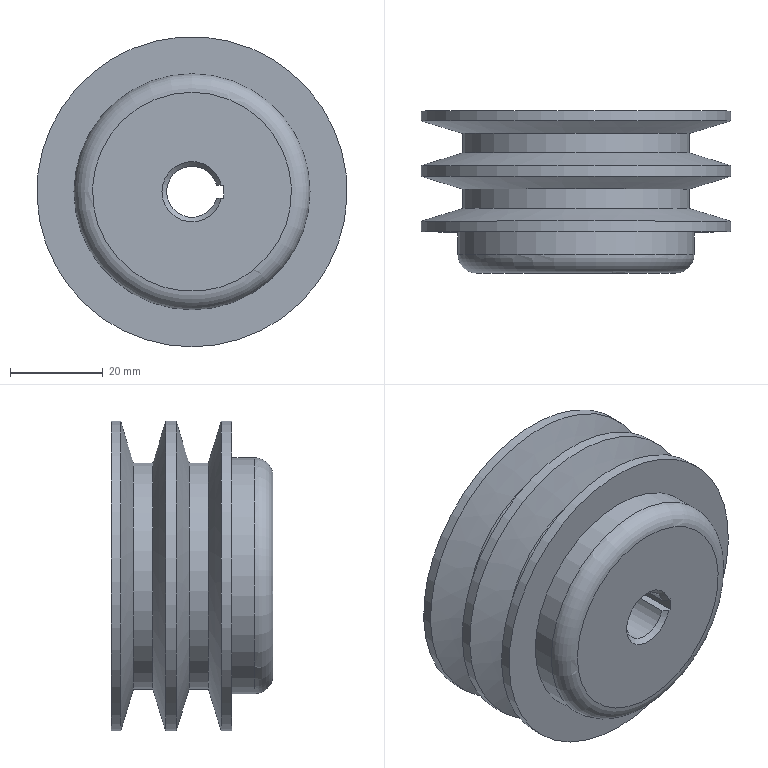Part | NX | features DATUM_CSYS 3, SKETCH 2, BLEND 1, CHAMFER 1, EXTRUDE 1, SWP104 1 | 1 solid | 20 faces | box 67 x 35 x 67 mm | volume 82909 mm3 | cylinder 7 | plane 6 | cone 6 | torus 1 | commonest cylinder face diameters 67 x3 49 x2 11 x1 51 x1
STEP:
#1=CARTESIAN_POINT('',(0.,0.,21.5));
#2=VERTEX_POINT('',#1);
#3=CARTESIAN_POINT('',(0.,0.,0.));
#4=DIRECTION('',(0.,1.,0.));
#5=DIRECTION('',(0.,0.,1.));
#6=AXIS2_PLACEMENT_3D('',#3,#4,#5);
#7=CIRCLE('',#6,21.5);
#8=EDGE_CURVE('',#2,#2,#7,.F.);
#9=ORIENTED_EDGE('',*,*,#8,.T.);
#10=EDGE_LOOP('',(#9));
#11=FACE_BOUND('',#10,.T.);
#12=CARTESIAN_POINT('',(6.347,0.,-1.4));
#13=VERTEX_POINT('',#12);
#14=CARTESIAN_POINT('',(6.9,0.,-1.4));
#15=VERTEX_POINT('',#14);
#16=CARTESIAN_POINT('',(0.,0.,-1.4));
#17=DIRECTION('',(1.,0.,0.));
#18=VECTOR('',#17,1000.);
#19=LINE('',#16,#18);
#20=EDGE_CURVE('',#13,#15,#19,.T.);
#21=ORIENTED_EDGE('',*,*,#20,.F.);
#22=CARTESIAN_POINT('',(6.347,0.,1.4));
#23=VERTEX_POINT('',#22);
#24=CARTESIAN_POINT('',(0.,0.,0.));
#25=DIRECTION('',(0.,1.,0.));
#26=DIRECTION('',(0.,0.,1.));
#27=AXIS2_PLACEMENT_3D('',#24,#25,#26);
#28=CIRCLE('',#27,6.5);
#29=EDGE_CURVE('',#13,#23,#28,.T.);
#30=ORIENTED_EDGE('',*,*,#29,.T.);
#31=CARTESIAN_POINT('',(6.9,0.,1.4));
#32=VERTEX_POINT('',#31);
#33=CARTESIAN_POINT('',(0.,0.,1.4));
#34=DIRECTION('',(-1.,0.,0.));
#35=VECTOR('',#34,1000.);
#36=LINE('',#33,#35);
#37=EDGE_CURVE('',#32,#23,#36,.T.);
#38=ORIENTED_EDGE('',*,*,#37,.F.);
#39=CARTESIAN_POINT('',(6.9,0.,25.5));
#40=DIRECTION('',(0.,0.,1.));
#41=VECTOR('',#40,1000.);
#42=LINE('',#39,#41);
#43=EDGE_CURVE('',#15,#32,#42,.T.);
#44=ORIENTED_EDGE('',*,*,#43,.F.);
#45=EDGE_LOOP('',(#21,#30,#38,#44));
#46=FACE_BOUND('',#45,.T.);
#47=CARTESIAN_POINT('',(0.,0.,25.5));
#48=DIRECTION('',(0.,1.,0.));
#49=DIRECTION('',(0.,0.,1.));
#50=AXIS2_PLACEMENT_3D('',#47,#48,#49);
#51=PLANE('',#50);
#52=ADVANCED_FACE('',(#11,#46),#51,.F.);
#53=CARTESIAN_POINT('',(5.319,34.,-1.4));
#54=VERTEX_POINT('',#53);
#55=CARTESIAN_POINT('',(5.319,1.,-1.4));
#56=VERTEX_POINT('',#55);
#57=CARTESIAN_POINT('',(5.319,0.,-1.4));
#58=DIRECTION('',(0.,-1.,0.));
#59=VECTOR('',#58,1000.);
#60=LINE('',#57,#59);
#61=EDGE_CURVE('',#54,#56,#60,.T.);
#62=ORIENTED_EDGE('',*,*,#61,.F.);
#63=CARTESIAN_POINT('',(5.319,34.,1.4));
#64=VERTEX_POINT('',#63);
#65=CARTESIAN_POINT('',(0.,34.,0.));
#66=DIRECTION('',(0.,-1.,0.));
#67=DIRECTION('',(0.,0.,-1.));
#68=AXIS2_PLACEMENT_3D('',#65,#66,#67);
#69=CIRCLE('',#68,5.5);
#70=EDGE_CURVE('',#54,#64,#69,.F.);
#71=ORIENTED_EDGE('',*,*,#70,.T.);
#72=CARTESIAN_POINT('',(5.319,1.,1.4));
#73=VERTEX_POINT('',#72);
#74=CARTESIAN_POINT('',(5.319,0.,1.4));
#75=DIRECTION('',(0.,-1.,0.));
#76=VECTOR('',#75,1000.);
#77=LINE('',#74,#76);
#78=EDGE_CURVE('',#73,#64,#77,.F.);
#79=ORIENTED_EDGE('',*,*,#78,.F.);
#80=CARTESIAN_POINT('',(0.,1.,0.));
#81=DIRECTION('',(0.,1.,0.));
#82=DIRECTION('',(0.,0.,1.));
#83=AXIS2_PLACEMENT_3D('',#80,#81,#82);
#84=CIRCLE('',#83,5.5);
#85=EDGE_CURVE('',#73,#56,#84,.F.);
#86=ORIENTED_EDGE('',*,*,#85,.T.);
#87=EDGE_LOOP('',(#62,#71,#79,#86));
#88=FACE_BOUND('',#87,.T.);
#89=CARTESIAN_POINT('',(0.,0.,0.));
#90=DIRECTION('',(0.,-1.,0.));
#91=DIRECTION('',(0.,0.,-1.));
#92=AXIS2_PLACEMENT_3D('',#89,#90,#91);
#93=CYLINDRICAL_SURFACE('',#92,5.5);
#94=ADVANCED_FACE('',(#88),#93,.F.);
#95=CARTESIAN_POINT('',(0.,35.,-33.5));
#96=VERTEX_POINT('',#95);
#97=CARTESIAN_POINT('',(0.,35.,0.));
#98=DIRECTION('',(0.,-1.,0.));
#99=DIRECTION('',(0.,0.,-1.));
#100=AXIS2_PLACEMENT_3D('',#97,#98,#99);
#101=CIRCLE('',#100,33.5);
#102=EDGE_CURVE('',#96,#96,#101,.T.);
#103=ORIENTED_EDGE('',*,*,#102,.F.);
#104=EDGE_LOOP('',(#103));
#105=FACE_BOUND('',#104,.T.);
#106=CARTESIAN_POINT('',(6.347,35.,1.4));
#107=VERTEX_POINT('',#106);
#108=CARTESIAN_POINT('',(6.9,35.,1.4));
#109=VERTEX_POINT('',#108);
#110=CARTESIAN_POINT('',(0.,35.,1.4));
#111=DIRECTION('',(1.,0.,0.));
#112=VECTOR('',#111,1000.);
#113=LINE('',#110,#112);
#114=EDGE_CURVE('',#107,#109,#113,.T.);
#115=ORIENTED_EDGE('',*,*,#114,.F.);
#116=CARTESIAN_POINT('',(6.347,35.,-1.4));
#117=VERTEX_POINT('',#116);
#118=CARTESIAN_POINT('',(0.,35.,0.));
#119=DIRECTION('',(0.,-1.,0.));
#120=DIRECTION('',(0.,0.,-1.));
#121=AXIS2_PLACEMENT_3D('',#118,#119,#120);
#122=CIRCLE('',#121,6.5);
#123=EDGE_CURVE('',#107,#117,#122,.T.);
#124=ORIENTED_EDGE('',*,*,#123,.T.);
#125=CARTESIAN_POINT('',(6.9,35.,-1.4));
#126=VERTEX_POINT('',#125);
#127=CARTESIAN_POINT('',(0.,35.,-1.4));
#128=DIRECTION('',(-1.,0.,0.));
#129=VECTOR('',#128,1000.);
#130=LINE('',#127,#129);
#131=EDGE_CURVE('',#126,#117,#130,.T.);
#132=ORIENTED_EDGE('',*,*,#131,.F.);
#133=CARTESIAN_POINT('',(6.9,35.,5.5));
#134=DIRECTION('',(0.,0.,-1.));
#135=VECTOR('',#134,1000.);
#136=LINE('',#133,#135);
#137=EDGE_CURVE('',#109,#126,#136,.T.);
#138=ORIENTED_EDGE('',*,*,#137,.F.);
#139=EDGE_LOOP('',(#115,#124,#132,#138));
#140=FACE_BOUND('',#139,.T.);
#141=CARTESIAN_POINT('',(0.,35.,5.5));
#142=DIRECTION('',(0.,-1.,0.));
#143=DIRECTION('',(0.,0.,-1.));
#144=AXIS2_PLACEMENT_3D('',#141,#142,#143);
#145=PLANE('',#144);
#146=ADVANCED_FACE('',(#105,#140),#145,.F.);
#147=CARTESIAN_POINT('',(0.,32.9,-33.5));
#148=VERTEX_POINT('',#147);
#149=CARTESIAN_POINT('',(0.,32.9,0.));
#150=DIRECTION('',(0.,-1.,0.));
#151=DIRECTION('',(0.,0.,-1.));
#152=AXIS2_PLACEMENT_3D('',#149,#150,#151);
#153=CIRCLE('',#152,33.5);
#154=EDGE_CURVE('',#148,#148,#153,.T.);
#155=ORIENTED_EDGE('',*,*,#154,.F.);
#156=EDGE_LOOP('',(#155));
#157=FACE_BOUND('',#156,.T.);
#158=ORIENTED_EDGE('',*,*,#102,.T.);
#159=EDGE_LOOP('',(#158));
#160=FACE_BOUND('',#159,.T.);
#161=CARTESIAN_POINT('',(0.,0.,0.));
#162=DIRECTION('',(0.,-1.,0.));
#163=DIRECTION('',(0.,0.,-1.));
#164=AXIS2_PLACEMENT_3D('',#161,#162,#163);
#165=CYLINDRICAL_SURFACE('',#164,33.5);
#166=ADVANCED_FACE('',(#157,#160),#165,.T.);
#167=CARTESIAN_POINT('',(0.,30.148,-24.5));
#168=VERTEX_POINT('',#167);
#169=CARTESIAN_POINT('',(0.,30.148,0.));
#170=DIRECTION('',(0.,-1.,0.));
#171=DIRECTION('',(0.,0.,-1.));
#172=AXIS2_PLACEMENT_3D('',#169,#170,#171);
#173=CIRCLE('',#172,24.5);
#174=EDGE_CURVE('',#168,#168,#173,.T.);
#175=ORIENTED_EDGE('',*,*,#174,.F.);
#176=EDGE_LOOP('',(#175));
#177=FACE_BOUND('',#176,.T.);
#178=ORIENTED_EDGE('',*,*,#154,.T.);
#179=EDGE_LOOP('',(#178));
#180=FACE_BOUND('',#179,.T.);
#181=CARTESIAN_POINT('',(0.,32.9,0.));
#182=DIRECTION('',(0.,1.,0.));
#183=DIRECTION('',(0.,0.,1.));
#184=AXIS2_PLACEMENT_3D('',#181,#182,#183);
#185=CONICAL_SURFACE('',#184,33.5,1.274);
#186=ADVANCED_FACE('',(#177,#180),#185,.T.);
#187=CARTESIAN_POINT('',(0.,25.948,-24.5));
#188=VERTEX_POINT('',#187);
#189=CARTESIAN_POINT('',(0.,25.948,0.));
#190=DIRECTION('',(0.,-1.,0.));
#191=DIRECTION('',(0.,0.,-1.));
#192=AXIS2_PLACEMENT_3D('',#189,#190,#191);
#193=CIRCLE('',#192,24.5);
#194=EDGE_CURVE('',#188,#188,#193,.T.);
#195=ORIENTED_EDGE('',*,*,#194,.F.);
#196=EDGE_LOOP('',(#195));
#197=FACE_BOUND('',#196,.T.);
#198=ORIENTED_EDGE('',*,*,#174,.T.);
#199=EDGE_LOOP('',(#198));
#200=FACE_BOUND('',#199,.T.);
#201=CARTESIAN_POINT('',(0.,0.,0.));
#202=DIRECTION('',(0.,-1.,0.));
#203=DIRECTION('',(0.,0.,-1.));
#204=AXIS2_PLACEMENT_3D('',#201,#202,#203);
#205=CYLINDRICAL_SURFACE('',#204,24.5);
#206=ADVANCED_FACE('',(#197,#200),#205,.T.);
#207=CARTESIAN_POINT('',(0.,23.197,-33.5));
#208=VERTEX_POINT('',#207);
#209=CARTESIAN_POINT('',(0.,23.197,0.));
#210=DIRECTION('',(0.,-1.,0.));
#211=DIRECTION('',(0.,0.,-1.));
#212=AXIS2_PLACEMENT_3D('',#209,#210,#211);
#213=CIRCLE('',#212,33.5);
#214=EDGE_CURVE('',#208,#208,#213,.T.);
#215=ORIENTED_EDGE('',*,*,#214,.F.);
#216=EDGE_LOOP('',(#215));
#217=FACE_BOUND('',#216,.T.);
#218=ORIENTED_EDGE('',*,*,#194,.T.);
#219=EDGE_LOOP('',(#218));
#220=FACE_BOUND('',#219,.T.);
#221=CARTESIAN_POINT('',(0.,25.948,0.));
#222=DIRECTION('',(0.,-1.,0.));
#223=DIRECTION('',(0.,0.,-1.));
#224=AXIS2_PLACEMENT_3D('',#221,#222,#223);
#225=CONICAL_SURFACE('',#224,24.5,1.274);
#226=ADVANCED_FACE('',(#217,#220),#225,.T.);
#227=CARTESIAN_POINT('',(0.,20.897,-33.5));
#228=VERTEX_POINT('',#227);
#229=CARTESIAN_POINT('',(0.,20.897,0.));
#230=DIRECTION('',(0.,-1.,0.));
#231=DIRECTION('',(0.,0.,-1.));
#232=AXIS2_PLACEMENT_3D('',#229,#230,#231);
#233=CIRCLE('',#232,33.5);
#234=EDGE_CURVE('',#228,#228,#233,.T.);
#235=ORIENTED_EDGE('',*,*,#234,.F.);
#236=EDGE_LOOP('',(#235));
#237=FACE_BOUND('',#236,.T.);
#238=ORIENTED_EDGE('',*,*,#214,.T.);
#239=EDGE_LOOP('',(#238));
#240=FACE_BOUND('',#239,.T.);
#241=CARTESIAN_POINT('',(0.,0.,0.));
#242=DIRECTION('',(0.,-1.,0.));
#243=DIRECTION('',(0.,0.,-1.));
#244=AXIS2_PLACEMENT_3D('',#241,#242,#243);
#245=CYLINDRICAL_SURFACE('',#244,33.5);
#246=ADVANCED_FACE('',(#237,#240),#245,.T.);
#247=CARTESIAN_POINT('',(0.,18.145,-24.5));
#248=VERTEX_POINT('',#247);
#249=CARTESIAN_POINT('',(0.,18.145,0.));
#250=DIRECTION('',(0.,-1.,0.));
#251=DIRECTION('',(0.,0.,-1.));
#252=AXIS2_PLACEMENT_3D('',#249,#250,#251);
#253=CIRCLE('',#252,24.5);
#254=EDGE_CURVE('',#248,#248,#253,.T.);
#255=ORIENTED_EDGE('',*,*,#254,.F.);
#256=EDGE_LOOP('',(#255));
#257=FACE_BOUND('',#256,.T.);
#258=ORIENTED_EDGE('',*,*,#234,.T.);
#259=EDGE_LOOP('',(#258));
#260=FACE_BOUND('',#259,.T.);
#261=CARTESIAN_POINT('',(0.,20.897,0.));
#262=DIRECTION('',(0.,1.,0.));
#263=DIRECTION('',(0.,0.,1.));
#264=AXIS2_PLACEMENT_3D('',#261,#262,#263);
#265=CONICAL_SURFACE('',#264,33.5,1.274);
#266=ADVANCED_FACE('',(#257,#260),#265,.T.);
#267=CARTESIAN_POINT('',(0.,13.945,-24.5));
#268=VERTEX_POINT('',#267);
#269=CARTESIAN_POINT('',(0.,13.945,0.));
#270=DIRECTION('',(0.,-1.,0.));
#271=DIRECTION('',(0.,0.,-1.));
#272=AXIS2_PLACEMENT_3D('',#269,#270,#271);
#273=CIRCLE('',#272,24.5);
#274=EDGE_CURVE('',#268,#268,#273,.T.);
#275=ORIENTED_EDGE('',*,*,#274,.F.);
#276=EDGE_LOOP('',(#275));
#277=FACE_BOUND('',#276,.T.);
#278=ORIENTED_EDGE('',*,*,#254,.T.);
#279=EDGE_LOOP('',(#278));
#280=FACE_BOUND('',#279,.T.);
#281=CARTESIAN_POINT('',(0.,0.,0.));
#282=DIRECTION('',(0.,-1.,0.));
#283=DIRECTION('',(0.,0.,-1.));
#284=AXIS2_PLACEMENT_3D('',#281,#282,#283);
#285=CYLINDRICAL_SURFACE('',#284,24.5);
#286=ADVANCED_FACE('',(#277,#280),#285,.T.);
#287=CARTESIAN_POINT('',(0.,11.194,-33.5));
#288=VERTEX_POINT('',#287);
#289=CARTESIAN_POINT('',(0.,11.194,0.));
#290=DIRECTION('',(0.,-1.,0.));
#291=DIRECTION('',(0.,0.,-1.));
#292=AXIS2_PLACEMENT_3D('',#289,#290,#291);
#293=CIRCLE('',#292,33.5);
#294=EDGE_CURVE('',#288,#288,#293,.T.);
#295=ORIENTED_EDGE('',*,*,#294,.F.);
#296=EDGE_LOOP('',(#295));
#297=FACE_BOUND('',#296,.T.);
#298=ORIENTED_EDGE('',*,*,#274,.T.);
#299=EDGE_LOOP('',(#298));
#300=FACE_BOUND('',#299,.T.);
#301=CARTESIAN_POINT('',(0.,13.945,0.));
#302=DIRECTION('',(0.,-1.,0.));
#303=DIRECTION('',(0.,0.,-1.));
#304=AXIS2_PLACEMENT_3D('',#301,#302,#303);
#305=CONICAL_SURFACE('',#304,24.5,1.274);
#306=ADVANCED_FACE('',(#297,#300),#305,.T.);
#307=CARTESIAN_POINT('',(0.,8.894,-33.5));
#308=VERTEX_POINT('',#307);
#309=CARTESIAN_POINT('',(0.,8.894,0.));
#310=DIRECTION('',(0.,-1.,0.));
#311=DIRECTION('',(0.,0.,-1.));
#312=AXIS2_PLACEMENT_3D('',#309,#310,#311);
#313=CIRCLE('',#312,33.5);
#314=EDGE_CURVE('',#308,#308,#313,.T.);
#315=ORIENTED_EDGE('',*,*,#314,.F.);
#316=EDGE_LOOP('',(#315));
#317=FACE_BOUND('',#316,.T.);
#318=ORIENTED_EDGE('',*,*,#294,.T.);
#319=EDGE_LOOP('',(#318));
#320=FACE_BOUND('',#319,.T.);
#321=CARTESIAN_POINT('',(0.,0.,0.));
#322=DIRECTION('',(0.,-1.,0.));
#323=DIRECTION('',(0.,0.,-1.));
#324=AXIS2_PLACEMENT_3D('',#321,#322,#323);
#325=CYLINDRICAL_SURFACE('',#324,33.5);
#326=ADVANCED_FACE('',(#317,#320),#325,.T.);
#327=CARTESIAN_POINT('',(0.,8.894,-25.5));
#328=VERTEX_POINT('',#327);
#329=CARTESIAN_POINT('',(0.,8.894,0.));
#330=DIRECTION('',(0.,-1.,0.));
#331=DIRECTION('',(0.,0.,-1.));
#332=AXIS2_PLACEMENT_3D('',#329,#330,#331);
#333=CIRCLE('',#332,25.5);
#334=EDGE_CURVE('',#328,#328,#333,.T.);
#335=ORIENTED_EDGE('',*,*,#334,.F.);
#336=EDGE_LOOP('',(#335));
#337=FACE_BOUND('',#336,.T.);
#338=ORIENTED_EDGE('',*,*,#314,.T.);
#339=EDGE_LOOP('',(#338));
#340=FACE_BOUND('',#339,.T.);
#341=CARTESIAN_POINT('',(0.,8.894,33.5));
#342=DIRECTION('',(0.,1.,0.));
#343=DIRECTION('',(0.,0.,1.));
#344=AXIS2_PLACEMENT_3D('',#341,#342,#343);
#345=PLANE('',#344);
#346=ADVANCED_FACE('',(#337,#340),#345,.F.);
#347=CARTESIAN_POINT('',(0.,4.,25.5));
#348=VERTEX_POINT('',#347);
#349=CARTESIAN_POINT('',(0.,4.,0.));
#350=DIRECTION('',(0.,1.,0.));
#351=DIRECTION('',(0.,0.,1.));
#352=AXIS2_PLACEMENT_3D('',#349,#350,#351);
#353=CIRCLE('',#352,25.5);
#354=EDGE_CURVE('',#348,#348,#353,.T.);
#355=ORIENTED_EDGE('',*,*,#354,.T.);
#356=EDGE_LOOP('',(#355));
#357=FACE_BOUND('',#356,.T.);
#358=ORIENTED_EDGE('',*,*,#334,.T.);
#359=EDGE_LOOP('',(#358));
#360=FACE_BOUND('',#359,.T.);
#361=CARTESIAN_POINT('',(0.,0.,0.));
#362=DIRECTION('',(0.,-1.,0.));
#363=DIRECTION('',(0.,0.,-1.));
#364=AXIS2_PLACEMENT_3D('',#361,#362,#363);
#365=CYLINDRICAL_SURFACE('',#364,25.5);
#366=ADVANCED_FACE('',(#357,#360),#365,.T.);
#367=ORIENTED_EDGE('',*,*,#78,.T.);
#368=CARTESIAN_POINT('',(5.319,34.,1.4));
#369=CARTESIAN_POINT('',(5.663,34.332,1.4));
#370=CARTESIAN_POINT('',(6.005,34.666,1.4));
#371=CARTESIAN_POINT('',(6.347,35.,1.4));
#372=B_SPLINE_CURVE_WITH_KNOTS('',3,(#368,#369,#370,#371),.UNSPECIFIED.,.F.,.F.,(4,4),(0.,0.001435),.UNSPECIFIED.);
#373=EDGE_CURVE('',#64,#107,#372,.T.);
#374=ORIENTED_EDGE('',*,*,#373,.T.);
#375=ORIENTED_EDGE('',*,*,#114,.T.);
#376=CARTESIAN_POINT('',(6.9,109.,1.4));
#377=DIRECTION('',(0.,-1.,0.));
#378=VECTOR('',#377,1000.);
#379=LINE('',#376,#378);
#380=EDGE_CURVE('',#32,#109,#379,.F.);
#381=ORIENTED_EDGE('',*,*,#380,.F.);
#382=ORIENTED_EDGE('',*,*,#37,.T.);
#383=CARTESIAN_POINT('',(6.347,0.,1.4));
#384=CARTESIAN_POINT('',(6.005,0.3341,1.4));
#385=CARTESIAN_POINT('',(5.663,0.6676,1.4));
#386=CARTESIAN_POINT('',(5.319,1.,1.4));
#387=B_SPLINE_CURVE_WITH_KNOTS('',3,(#383,#384,#385,#386),.UNSPECIFIED.,.F.,.F.,(4,4),(0.,0.001435),.UNSPECIFIED.);
#388=EDGE_CURVE('',#23,#73,#387,.T.);
#389=ORIENTED_EDGE('',*,*,#388,.T.);
#390=EDGE_LOOP('',(#367,#374,#375,#381,#382,#389));
#391=FACE_BOUND('',#390,.T.);
#392=CARTESIAN_POINT('',(4.1,109.,1.4));
#393=DIRECTION('',(0.,0.,-1.));
#394=DIRECTION('',(-1.,0.,0.));
#395=AXIS2_PLACEMENT_3D('',#392,#393,#394);
#396=PLANE('',#395);
#397=ADVANCED_FACE('',(#391),#396,.T.);
#398=ORIENTED_EDGE('',*,*,#43,.T.);
#399=ORIENTED_EDGE('',*,*,#380,.T.);
#400=ORIENTED_EDGE('',*,*,#137,.T.);
#401=CARTESIAN_POINT('',(6.9,109.,-1.4));
#402=DIRECTION('',(0.,-1.,0.));
#403=VECTOR('',#402,1000.);
#404=LINE('',#401,#403);
#405=EDGE_CURVE('',#15,#126,#404,.F.);
#406=ORIENTED_EDGE('',*,*,#405,.F.);
#407=EDGE_LOOP('',(#398,#399,#400,#406));
#408=FACE_BOUND('',#407,.T.);
#409=CARTESIAN_POINT('',(6.9,109.,1.4));
#410=DIRECTION('',(-1.,0.,0.));
#411=DIRECTION('',(0.,0.,1.));
#412=AXIS2_PLACEMENT_3D('',#409,#410,#411);
#413=PLANE('',#412);
#414=ADVANCED_FACE('',(#408),#413,.T.);
#415=ORIENTED_EDGE('',*,*,#131,.T.);
#416=CARTESIAN_POINT('',(6.347,35.,-1.4));
#417=CARTESIAN_POINT('',(6.005,34.666,-1.4));
#418=CARTESIAN_POINT('',(5.663,34.332,-1.4));
#419=CARTESIAN_POINT('',(5.319,34.,-1.4));
#420=B_SPLINE_CURVE_WITH_KNOTS('',3,(#416,#417,#418,#419),.UNSPECIFIED.,.F.,.F.,(4,4),(0.,0.001435),.UNSPECIFIED.);
#421=EDGE_CURVE('',#117,#54,#420,.T.);
#422=ORIENTED_EDGE('',*,*,#421,.T.);
#423=ORIENTED_EDGE('',*,*,#61,.T.);
#424=CARTESIAN_POINT('',(5.319,1.,-1.4));
#425=CARTESIAN_POINT('',(5.663,0.6676,-1.4));
#426=CARTESIAN_POINT('',(6.005,0.3341,-1.4));
#427=CARTESIAN_POINT('',(6.347,0.,-1.4));
#428=B_SPLINE_CURVE_WITH_KNOTS('',3,(#424,#425,#426,#427),.UNSPECIFIED.,.F.,.F.,(4,4),(0.,0.001435),.UNSPECIFIED.);
#429=EDGE_CURVE('',#56,#13,#428,.T.);
#430=ORIENTED_EDGE('',*,*,#429,.T.);
#431=ORIENTED_EDGE('',*,*,#20,.T.);
#432=ORIENTED_EDGE('',*,*,#405,.T.);
#433=EDGE_LOOP('',(#415,#422,#423,#430,#431,#432));
#434=FACE_BOUND('',#433,.T.);
#435=CARTESIAN_POINT('',(6.9,109.,-1.4));
#436=DIRECTION('',(0.,0.,1.));
#437=DIRECTION('',(1.,0.,0.));
#438=AXIS2_PLACEMENT_3D('',#435,#436,#437);
#439=PLANE('',#438);
#440=ADVANCED_FACE('',(#434),#439,.T.);
#441=ORIENTED_EDGE('',*,*,#354,.F.);
#442=EDGE_LOOP('',(#441));
#443=FACE_BOUND('',#442,.T.);
#444=ORIENTED_EDGE('',*,*,#8,.F.);
#445=EDGE_LOOP('',(#444));
#446=FACE_BOUND('',#445,.T.);
#447=CARTESIAN_POINT('',(0.,4.,0.));
#448=DIRECTION('',(0.,1.,0.));
#449=DIRECTION('',(0.,0.,1.));
#450=AXIS2_PLACEMENT_3D('',#447,#448,#449);
#451=TOROIDAL_SURFACE('',#450,21.5,4.);
#452=ADVANCED_FACE('',(#443,#446),#451,.T.);
#453=ORIENTED_EDGE('',*,*,#373,.F.);
#454=ORIENTED_EDGE('',*,*,#70,.F.);
#455=ORIENTED_EDGE('',*,*,#421,.F.);
#456=ORIENTED_EDGE('',*,*,#123,.F.);
#457=EDGE_LOOP('',(#453,#454,#455,#456));
#458=FACE_BOUND('',#457,.T.);
#459=CARTESIAN_POINT('',(0.,35.,0.));
#460=DIRECTION('',(0.,1.,0.));
#461=DIRECTION('',(0.,0.,1.));
#462=AXIS2_PLACEMENT_3D('',#459,#460,#461);
#463=CONICAL_SURFACE('',#462,6.5,0.7854);
#464=ADVANCED_FACE('',(#458),#463,.F.);
#465=ORIENTED_EDGE('',*,*,#388,.F.);
#466=ORIENTED_EDGE('',*,*,#29,.F.);
#467=ORIENTED_EDGE('',*,*,#429,.F.);
#468=ORIENTED_EDGE('',*,*,#85,.F.);
#469=EDGE_LOOP('',(#465,#466,#467,#468));
#470=FACE_BOUND('',#469,.T.);
#471=CARTESIAN_POINT('',(0.,1.,0.));
#472=DIRECTION('',(0.,-1.,0.));
#473=DIRECTION('',(0.,0.,-1.));
#474=AXIS2_PLACEMENT_3D('',#471,#472,#473);
#475=CONICAL_SURFACE('',#474,5.5,0.7854);
#476=ADVANCED_FACE('',(#470),#475,.F.);
#477=CLOSED_SHELL('',(#52,#94,#146,#166,#186,#206,#226,#246,#266,#286,#306,#326,#346,#366,#397,#414,#440,#452,#464,#476));
#478=MANIFOLD_SOLID_BREP('',#477);
#479=(LENGTH_UNIT()NAMED_UNIT(*)SI_UNIT(.MILLI.,.METRE.));
#480=UNCERTAINTY_MEASURE_WITH_UNIT(LENGTH_MEASURE(0.0508),#479,'','');
#481=(NAMED_UNIT(*)PLANE_ANGLE_UNIT()SI_UNIT($,.RADIAN.));
#482=(NAMED_UNIT(*)SI_UNIT($,.STERADIAN.)SOLID_ANGLE_UNIT());
#483=(GEOMETRIC_REPRESENTATION_CONTEXT(3)GLOBAL_UNCERTAINTY_ASSIGNED_CONTEXT((#480))GLOBAL_UNIT_ASSIGNED_CONTEXT((#479,#481,#482))REPRESENTATION_CONTEXT('',''));
#484=ADVANCED_BREP_SHAPE_REPRESENTATION('',(#478),#483);